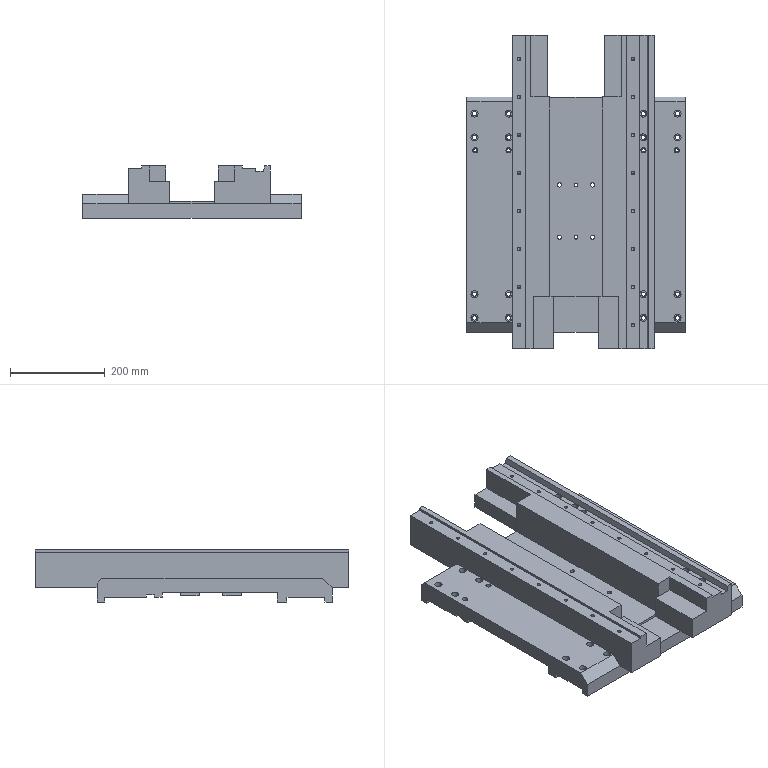Part | STEP file | 400V80 Main Carriage | 1 solid | 316 faces | box 460 x 660 x 110 mm | volume 11803093 mm3 | plane 160 | cylinder 124 | cone 32 | commonest cylinder face diameters 9 x40 6.8 x32 15 x32 7 x8 11 x8 8 x4